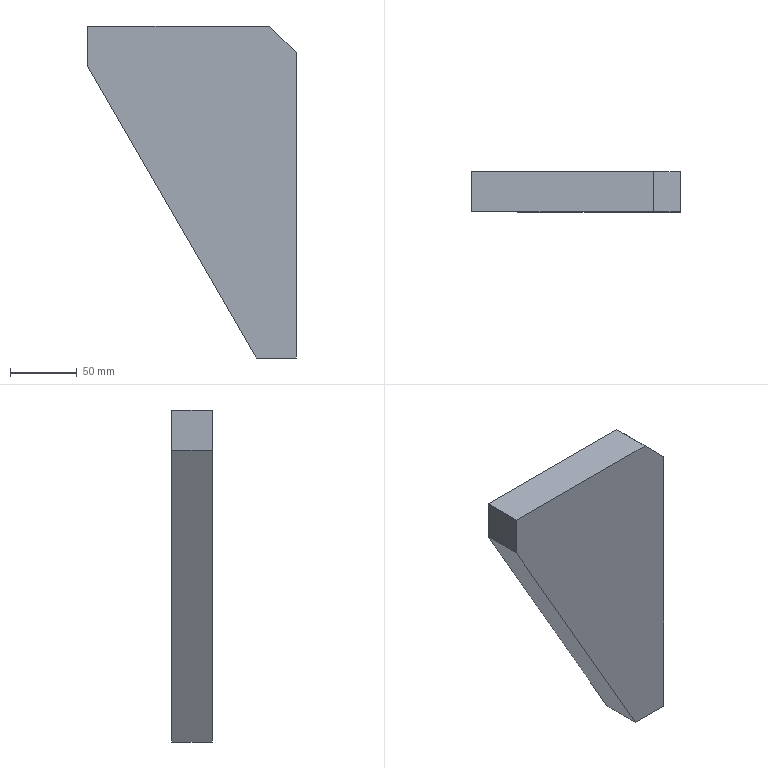Part | SolidWorks | features Extrusion 1 | 1 solid | 8 faces | box 155.862 x 30 x 248 mm | volume 742046 mm3 | plane 8
STEP:
#1=CARTESIAN_POINT('',(0.,0.,0.));
#2=VERTEX_POINT('',#1);
#3=CARTESIAN_POINT('',(-30.,0.,0.));
#4=VERTEX_POINT('',#3);
#5=CARTESIAN_POINT('',(-30.,0.,0.));
#6=DIRECTION('',(-1.,0.,0.));
#7=VECTOR('',#6,1000.);
#8=LINE('',#5,#7);
#9=EDGE_CURVE('',#2,#4,#8,.T.);
#10=ORIENTED_EDGE('',*,*,#9,.T.);
#11=CARTESIAN_POINT('',(-30.,30.,0.));
#12=VERTEX_POINT('',#11);
#13=CARTESIAN_POINT('',(-30.,30.,0.));
#14=DIRECTION('',(0.,-1.,0.));
#15=VECTOR('',#14,1000.);
#16=LINE('',#13,#15);
#17=EDGE_CURVE('',#12,#4,#16,.T.);
#18=ORIENTED_EDGE('',*,*,#17,.F.);
#19=CARTESIAN_POINT('',(0.,30.,0.));
#20=VERTEX_POINT('',#19);
#21=CARTESIAN_POINT('',(-30.,30.,0.));
#22=DIRECTION('',(-1.,0.,0.));
#23=VECTOR('',#22,1000.);
#24=LINE('',#21,#23);
#25=EDGE_CURVE('',#20,#12,#24,.T.);
#26=ORIENTED_EDGE('',*,*,#25,.F.);
#27=CARTESIAN_POINT('',(0.,30.,0.));
#28=DIRECTION('',(0.,-1.,0.));
#29=VECTOR('',#28,1000.);
#30=LINE('',#27,#29);
#31=EDGE_CURVE('',#20,#2,#30,.T.);
#32=ORIENTED_EDGE('',*,*,#31,.T.);
#33=EDGE_LOOP('',(#10,#18,#26,#32));
#34=FACE_OUTER_BOUND('',#33,.T.);
#35=CARTESIAN_POINT('',(-30.,30.,0.));
#36=DIRECTION('',(0.,0.,1.));
#37=DIRECTION('',(1.,0.,0.));
#38=AXIS2_PLACEMENT_3D('',#35,#36,#37);
#39=PLANE('',#38);
#40=ADVANCED_FACE('',(#34),#39,.F.);
#41=CARTESIAN_POINT('',(-155.862,0.,218.));
#42=VERTEX_POINT('',#41);
#43=CARTESIAN_POINT('',(-155.862,0.,218.));
#44=DIRECTION('',(-0.5,0.,0.866));
#45=VECTOR('',#44,1000.);
#46=LINE('',#43,#45);
#47=EDGE_CURVE('',#4,#42,#46,.T.);
#48=ORIENTED_EDGE('',*,*,#47,.T.);
#49=CARTESIAN_POINT('',(-155.862,30.,218.));
#50=VERTEX_POINT('',#49);
#51=CARTESIAN_POINT('',(-155.862,30.,218.));
#52=DIRECTION('',(0.,-1.,0.));
#53=VECTOR('',#52,1000.);
#54=LINE('',#51,#53);
#55=EDGE_CURVE('',#50,#42,#54,.T.);
#56=ORIENTED_EDGE('',*,*,#55,.F.);
#57=CARTESIAN_POINT('',(-155.862,30.,218.));
#58=DIRECTION('',(-0.5,0.,0.866));
#59=VECTOR('',#58,1000.);
#60=LINE('',#57,#59);
#61=EDGE_CURVE('',#12,#50,#60,.T.);
#62=ORIENTED_EDGE('',*,*,#61,.F.);
#63=ORIENTED_EDGE('',*,*,#17,.T.);
#64=EDGE_LOOP('',(#48,#56,#62,#63));
#65=FACE_OUTER_BOUND('',#64,.T.);
#66=CARTESIAN_POINT('',(-155.862,30.,218.));
#67=DIRECTION('',(0.866,0.,0.5));
#68=DIRECTION('',(0.5,0.,-0.866));
#69=AXIS2_PLACEMENT_3D('',#66,#67,#68);
#70=PLANE('',#69);
#71=ADVANCED_FACE('',(#65),#70,.F.);
#72=CARTESIAN_POINT('',(-155.862,0.,248.));
#73=VERTEX_POINT('',#72);
#74=CARTESIAN_POINT('',(-155.862,0.,248.));
#75=DIRECTION('',(0.,0.,1.));
#76=VECTOR('',#75,1000.);
#77=LINE('',#74,#76);
#78=EDGE_CURVE('',#42,#73,#77,.T.);
#79=ORIENTED_EDGE('',*,*,#78,.T.);
#80=CARTESIAN_POINT('',(-155.862,30.,248.));
#81=VERTEX_POINT('',#80);
#82=CARTESIAN_POINT('',(-155.862,30.,248.));
#83=DIRECTION('',(0.,-1.,0.));
#84=VECTOR('',#83,1000.);
#85=LINE('',#82,#84);
#86=EDGE_CURVE('',#81,#73,#85,.T.);
#87=ORIENTED_EDGE('',*,*,#86,.F.);
#88=CARTESIAN_POINT('',(-155.862,30.,248.));
#89=DIRECTION('',(0.,0.,1.));
#90=VECTOR('',#89,1000.);
#91=LINE('',#88,#90);
#92=EDGE_CURVE('',#50,#81,#91,.T.);
#93=ORIENTED_EDGE('',*,*,#92,.F.);
#94=ORIENTED_EDGE('',*,*,#55,.T.);
#95=EDGE_LOOP('',(#79,#87,#93,#94));
#96=FACE_OUTER_BOUND('',#95,.T.);
#97=CARTESIAN_POINT('',(-155.862,30.,248.));
#98=DIRECTION('',(1.,0.,0.));
#99=DIRECTION('',(0.,0.,-1.));
#100=AXIS2_PLACEMENT_3D('',#97,#98,#99);
#101=PLANE('',#100);
#102=ADVANCED_FACE('',(#96),#101,.F.);
#103=CARTESIAN_POINT('',(-20.,0.,248.));
#104=VERTEX_POINT('',#103);
#105=CARTESIAN_POINT('',(-20.,0.,248.));
#106=DIRECTION('',(1.,0.,0.));
#107=VECTOR('',#106,1000.);
#108=LINE('',#105,#107);
#109=EDGE_CURVE('',#73,#104,#108,.T.);
#110=ORIENTED_EDGE('',*,*,#109,.T.);
#111=CARTESIAN_POINT('',(-20.,30.,248.));
#112=VERTEX_POINT('',#111);
#113=CARTESIAN_POINT('',(-20.,30.,248.));
#114=DIRECTION('',(0.,-1.,0.));
#115=VECTOR('',#114,1000.);
#116=LINE('',#113,#115);
#117=EDGE_CURVE('',#112,#104,#116,.T.);
#118=ORIENTED_EDGE('',*,*,#117,.F.);
#119=CARTESIAN_POINT('',(-20.,30.,248.));
#120=DIRECTION('',(1.,0.,0.));
#121=VECTOR('',#120,1000.);
#122=LINE('',#119,#121);
#123=EDGE_CURVE('',#81,#112,#122,.T.);
#124=ORIENTED_EDGE('',*,*,#123,.F.);
#125=ORIENTED_EDGE('',*,*,#86,.T.);
#126=EDGE_LOOP('',(#110,#118,#124,#125));
#127=FACE_OUTER_BOUND('',#126,.T.);
#128=CARTESIAN_POINT('',(-20.,30.,248.));
#129=DIRECTION('',(0.,0.,-1.));
#130=DIRECTION('',(-1.,0.,0.));
#131=AXIS2_PLACEMENT_3D('',#128,#129,#130);
#132=PLANE('',#131);
#133=ADVANCED_FACE('',(#127),#132,.F.);
#134=CARTESIAN_POINT('',(0.,0.,228.));
#135=VERTEX_POINT('',#134);
#136=CARTESIAN_POINT('',(0.,0.,228.));
#137=DIRECTION('',(0.7071,0.,-0.7071));
#138=VECTOR('',#137,1000.);
#139=LINE('',#136,#138);
#140=EDGE_CURVE('',#104,#135,#139,.T.);
#141=ORIENTED_EDGE('',*,*,#140,.T.);
#142=CARTESIAN_POINT('',(0.,30.,228.));
#143=VERTEX_POINT('',#142);
#144=CARTESIAN_POINT('',(0.,30.,228.));
#145=DIRECTION('',(0.,-1.,0.));
#146=VECTOR('',#145,1000.);
#147=LINE('',#144,#146);
#148=EDGE_CURVE('',#143,#135,#147,.T.);
#149=ORIENTED_EDGE('',*,*,#148,.F.);
#150=CARTESIAN_POINT('',(0.,30.,228.));
#151=DIRECTION('',(0.7071,0.,-0.7071));
#152=VECTOR('',#151,1000.);
#153=LINE('',#150,#152);
#154=EDGE_CURVE('',#112,#143,#153,.T.);
#155=ORIENTED_EDGE('',*,*,#154,.F.);
#156=ORIENTED_EDGE('',*,*,#117,.T.);
#157=EDGE_LOOP('',(#141,#149,#155,#156));
#158=FACE_OUTER_BOUND('',#157,.T.);
#159=CARTESIAN_POINT('',(0.,30.,228.));
#160=DIRECTION('',(-0.7071,0.,-0.7071));
#161=DIRECTION('',(-0.7071,0.,0.7071));
#162=AXIS2_PLACEMENT_3D('',#159,#160,#161);
#163=PLANE('',#162);
#164=ADVANCED_FACE('',(#158),#163,.F.);
#165=CARTESIAN_POINT('',(0.,0.,0.));
#166=DIRECTION('',(0.,0.,-1.));
#167=VECTOR('',#166,1000.);
#168=LINE('',#165,#167);
#169=EDGE_CURVE('',#135,#2,#168,.T.);
#170=ORIENTED_EDGE('',*,*,#169,.T.);
#171=ORIENTED_EDGE('',*,*,#31,.F.);
#172=CARTESIAN_POINT('',(0.,30.,0.));
#173=DIRECTION('',(0.,0.,-1.));
#174=VECTOR('',#173,1000.);
#175=LINE('',#172,#174);
#176=EDGE_CURVE('',#143,#20,#175,.T.);
#177=ORIENTED_EDGE('',*,*,#176,.F.);
#178=ORIENTED_EDGE('',*,*,#148,.T.);
#179=EDGE_LOOP('',(#170,#171,#177,#178));
#180=FACE_OUTER_BOUND('',#179,.T.);
#181=CARTESIAN_POINT('',(0.,30.,0.));
#182=DIRECTION('',(-1.,0.,0.));
#183=DIRECTION('',(0.,0.,1.));
#184=AXIS2_PLACEMENT_3D('',#181,#182,#183);
#185=PLANE('',#184);
#186=ADVANCED_FACE('',(#180),#185,.F.);
#187=ORIENTED_EDGE('',*,*,#25,.T.);
#188=ORIENTED_EDGE('',*,*,#61,.T.);
#189=ORIENTED_EDGE('',*,*,#92,.T.);
#190=ORIENTED_EDGE('',*,*,#123,.T.);
#191=ORIENTED_EDGE('',*,*,#154,.T.);
#192=ORIENTED_EDGE('',*,*,#176,.T.);
#193=EDGE_LOOP('',(#187,#188,#189,#190,#191,#192));
#194=FACE_OUTER_BOUND('',#193,.T.);
#195=CARTESIAN_POINT('',(0.,30.,0.));
#196=DIRECTION('',(0.,-1.,0.));
#197=DIRECTION('',(0.,0.,-1.));
#198=AXIS2_PLACEMENT_3D('',#195,#196,#197);
#199=PLANE('',#198);
#200=ADVANCED_FACE('',(#194),#199,.F.);
#201=ORIENTED_EDGE('',*,*,#9,.F.);
#202=ORIENTED_EDGE('',*,*,#169,.F.);
#203=ORIENTED_EDGE('',*,*,#140,.F.);
#204=ORIENTED_EDGE('',*,*,#109,.F.);
#205=ORIENTED_EDGE('',*,*,#78,.F.);
#206=ORIENTED_EDGE('',*,*,#47,.F.);
#207=EDGE_LOOP('',(#201,#202,#203,#204,#205,#206));
#208=FACE_OUTER_BOUND('',#207,.T.);
#209=CARTESIAN_POINT('',(0.,0.,0.));
#210=DIRECTION('',(0.,-1.,0.));
#211=DIRECTION('',(0.,0.,-1.));
#212=AXIS2_PLACEMENT_3D('',#209,#210,#211);
#213=PLANE('',#212);
#214=ADVANCED_FACE('',(#208),#213,.T.);
#215=CLOSED_SHELL('',(#40,#71,#102,#133,#164,#186,#200,#214));
#216=MANIFOLD_SOLID_BREP('',#215);
#217=CARTESIAN_POINT('',(0.,0.,0.));
#218=DIRECTION('',(0.,0.,1.));
#219=DIRECTION('',(1.,0.,0.));
#220=AXIS2_PLACEMENT_3D('',#217,#218,#219);
#221=(LENGTH_UNIT()NAMED_UNIT(*)SI_UNIT(.MILLI.,.METRE.));
#222=UNCERTAINTY_MEASURE_WITH_UNIT(LENGTH_MEASURE(0.00001),#221,'','');
#223=(NAMED_UNIT(*)PLANE_ANGLE_UNIT()SI_UNIT($,.RADIAN.));
#224=(NAMED_UNIT(*)SI_UNIT($,.STERADIAN.)SOLID_ANGLE_UNIT());
#225=(GEOMETRIC_REPRESENTATION_CONTEXT(3)GLOBAL_UNCERTAINTY_ASSIGNED_CONTEXT((#222))GLOBAL_UNIT_ASSIGNED_CONTEXT((#221,#223,#224))REPRESENTATION_CONTEXT('',''));
#226=ADVANCED_BREP_SHAPE_REPRESENTATION('',(#216,#220),#225);